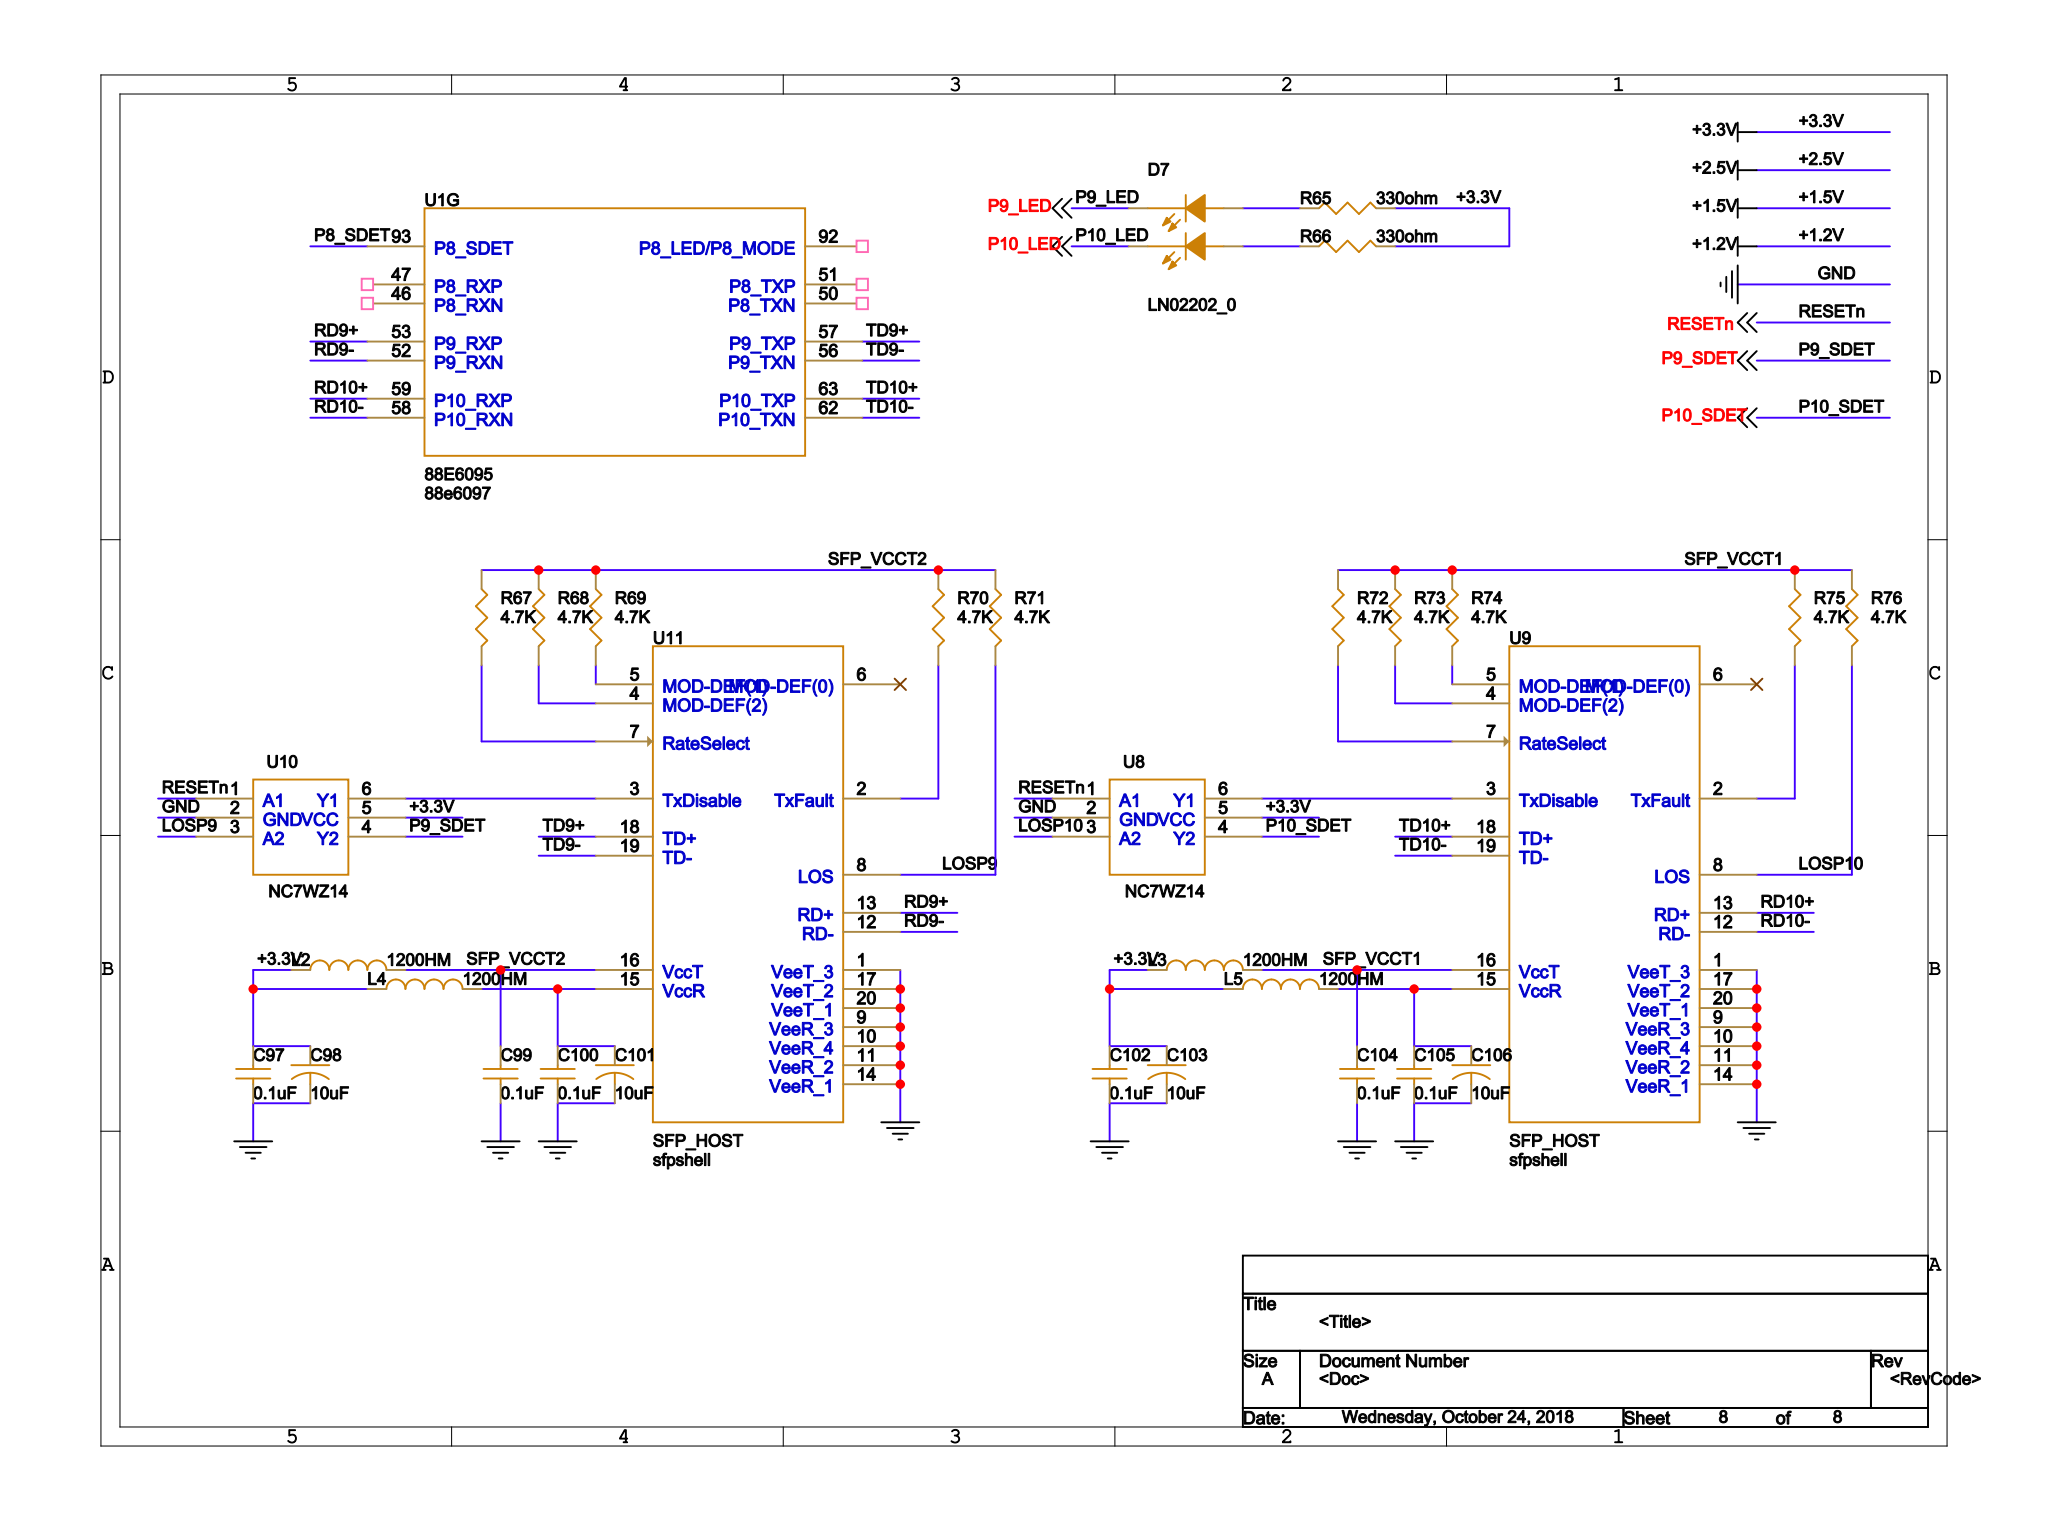Circuit board | Cadence Allegro | 219 parts | 174 nets | one sheet of the schematic
Parts on this sheet (reference | value | footprint):
C97 | 0.1uf | SC0603
C98 | 10uF | STC3528
C99 | 0.1uf | SC0603
C100 | 0.1uf | SC0603
C101 | 10uF | STC3528
C102 | 0.1uf | SC0603
C103 | 10uF | STC3528
C104 | 0.1uf | SC0603
C105 | 0.1uf | SC0603
C106 | 10uF | STC3528
D7 | LN02202_0 | LED_2
L2 | 1200HM | SL0805
L3 | 1200HM | SL0805
L4 | 1200HM | SL0805
L5 | 1200HM | SL0805
R65 | 330ohm | SR0603
R66 | 330ohm | SR0603
R67 | 4.7K | SR0603
R68 | 4.7K | SR0603
R69 | 4.7K | SR0603
R70 | 4.7K | SR0603
R71 | 4.7K | SR0603
R72 | 4.7K | SR0603
R73 | 4.7K | SR0603
R74 | 4.7K | SR0603
R75 | 4.7K | SR0603
R76 | 4.7K | SR0603
U1 | 88E6095 | 88E6097
U8 | NC7WZ14 | NC7W14
U9 | SFP_HOST | SFPSHELL
U10 | NC7WZ14 | NC7W14
U11 | SFP_HOST | SFPSHELL
Nets of these parts (net: part-pin ...):
GND: C97-2 C98-2 C99-2 C100-2 C101-2 C102-2 C103-2 C104-2 C105-2 C106-2 U8-2 U9-1 U9-9 U9-10 U9-11 U9-14 U9-17 U9-20 U10-2 U11-1 U11-9 U11-10 U11-11 U11-14 U11-17 U11-20
RESETN: U8-1 U10-1
P10_SDET: U8-4
P10_LED: D7-2
P9_SDET: U10-4
P9_LED: D7-4
+2.5V: U1-11
+1.2V: U1-3 U1-8 U1-14 U1-19
+3.3V: C97-1 C98-1 C102-1 C103-1 L2-1 L3-1 L4-1 L5-1 R65-2 R66-2 U8-5 U10-5
RD10-: U9-12 U1-58
RD10+: U9-13 U1-59
TD10-: U9-19 U1-62
TD10+: U9-18 U1-63
P8_SDET: U1-93
RD9-: U11-12 U1-52
RD9+: U11-13 U1-53
TD9-: U11-19 U1-56
TD9+: U11-18 U1-57
SFP_VCCT1: C104-1 L3-2 R72-1 R73-1 R74-1 R75-1 R76-1 U9-16
SFP_VCCT2: C99-1 L2-2 R67-1 R68-1 R69-1 R70-1 R71-1 U11-16
N1350879: C100-1 C101-1 L4-2 U11-15
N1351959: C105-1 C106-1 L5-2 U9-15
N1349774: D7-1 R66-1
N1349827: D7-3 R65-1
N1350498: R67-2 U11-7
N1350491: R68-2 U11-4
N1350549: R70-2 U11-2
N1350487: R69-2 U11-5
N1351777: R73-2 U9-4
N1351781: R74-2 U9-5
N1351785: R75-2 U9-2
LOSP10: R76-2 U8-3 U9-8
LOSP9: R71-2 U10-3 U11-8
N1351773: R72-2 U9-7
N1351538: U10-6 U11-3
N1351831: U8-6 U9-3